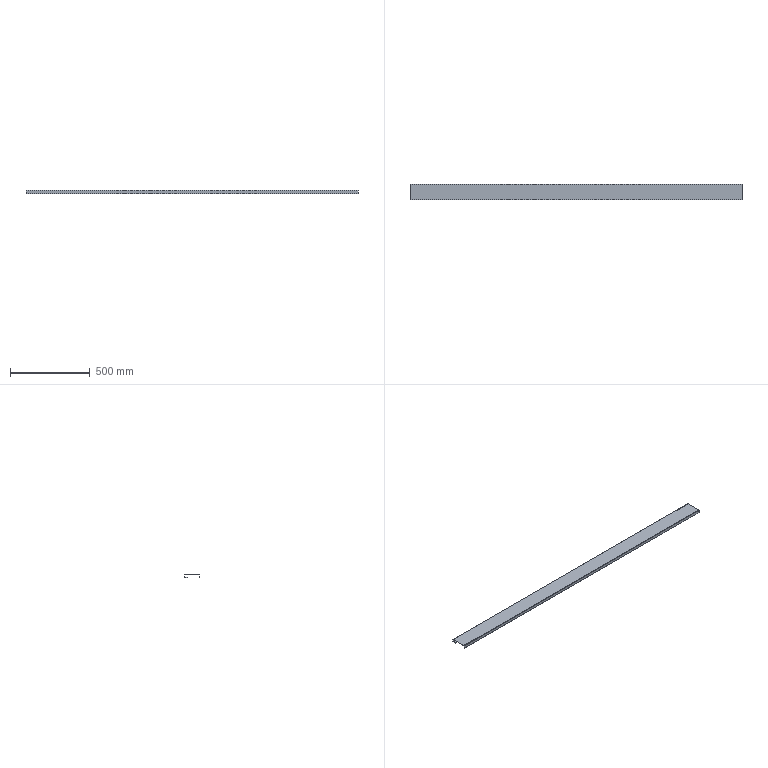Part | STEP file | E3-中转釜护栏3踢脚Plate | 1 solid | 18 faces | box 2088 x 100 x 20 mm | volume 479969 mm3 | plane 12 | cylinder 6 | commonest cylinder face diameters 2 x3 5 x3
STEP:
#1=CARTESIAN_POINT('',(0.,0.,0.));
#2=DIRECTION('',(0.,0.,1.));
#3=DIRECTION('',(1.,0.,0.));
#4=AXIS2_PLACEMENT_3D('',#1,#2,#3);
#5=CARTESIAN_POINT('',(-1044.,1.5,-2.5));
#6=VERTEX_POINT('',#5);
#7=CARTESIAN_POINT('',(-1044.,1.5,-20.));
#8=VERTEX_POINT('',#7);
#9=CARTESIAN_POINT('',(-1044.,1.5,-2.5));
#10=DIRECTION('',(0.,0.,-1.));
#11=VECTOR('',#10,1.);
#12=LINE('',#9,#11);
#13=CARTESIAN_POINT('',(1044.,1.5,-2.5));
#14=DIRECTION('',(0.,-1.,0.));
#15=DIRECTION('',(0.,0.,1.));
#16=AXIS2_PLACEMENT_3D('',#13,#14,#15);
#17=PLANE('',#16);
#18=CARTESIAN_POINT('',(0.,2088.));
#19=DIRECTION('',(-1.,0.));
#20=VECTOR('',#19,1.);
#21=LINE('',#18,#20);
#22=(GEOMETRIC_REPRESENTATION_CONTEXT(2)PARAMETRIC_REPRESENTATION_CONTEXT()REPRESENTATION_CONTEXT('',''));
#23=DEFINITIONAL_REPRESENTATION('',(#21),#22);
#24=PCURVE('',#17,#23);
#25=CARTESIAN_POINT('',(-1044.,2.5,-2.5));
#26=DIRECTION('',(-1.,0.,0.));
#27=DIRECTION('',(0.,0.,-1.));
#28=AXIS2_PLACEMENT_3D('',#25,#26,#27);
#29=PLANE('',#28);
#30=CARTESIAN_POINT('',(0.,1.));
#31=DIRECTION('',(1.,0.));
#32=VECTOR('',#31,1.);
#33=LINE('',#30,#32);
#34=(GEOMETRIC_REPRESENTATION_CONTEXT(2)PARAMETRIC_REPRESENTATION_CONTEXT()REPRESENTATION_CONTEXT('',''));
#35=DEFINITIONAL_REPRESENTATION('',(#33),#34);
#36=PCURVE('',#29,#35);
#37=SURFACE_CURVE('',#12,(#24,#36),.PCURVE_S1.);
#38=EDGE_CURVE('',#6,#8,#37,.T.);
#39=ORIENTED_EDGE('',*,*,#38,.F.);
#40=CARTESIAN_POINT('',(1044.,1.5,-2.5));
#41=VERTEX_POINT('',#40);
#42=CARTESIAN_POINT('',(1044.,1.5,-2.5));
#43=DIRECTION('',(-1.,0.,0.));
#44=VECTOR('',#43,1.);
#45=LINE('',#42,#44);
#46=CARTESIAN_POINT('',(0.,0.));
#47=DIRECTION('',(0.,1.));
#48=VECTOR('',#47,1.);
#49=LINE('',#46,#48);
#50=(GEOMETRIC_REPRESENTATION_CONTEXT(2)PARAMETRIC_REPRESENTATION_CONTEXT()REPRESENTATION_CONTEXT('',''));
#51=DEFINITIONAL_REPRESENTATION('',(#49),#50);
#52=PCURVE('',#17,#51);
#53=CARTESIAN_POINT('',(1044.,2.5,-2.5));
#54=DIRECTION('',(-1.,0.,0.));
#55=DIRECTION('',(0.,0.,-1.));
#56=AXIS2_PLACEMENT_3D('',#53,#54,#55);
#57=CYLINDRICAL_SURFACE('',#56,1.);
#58=CARTESIAN_POINT('',(1.571,0.));
#59=DIRECTION('',(0.,1.));
#60=VECTOR('',#59,1.);
#61=LINE('',#58,#60);
#62=(GEOMETRIC_REPRESENTATION_CONTEXT(2)PARAMETRIC_REPRESENTATION_CONTEXT()REPRESENTATION_CONTEXT('',''));
#63=DEFINITIONAL_REPRESENTATION('',(#61),#62);
#64=PCURVE('',#57,#63);
#65=SURFACE_CURVE('',#45,(#52,#64),.PCURVE_S1.);
#66=EDGE_CURVE('',#41,#6,#65,.T.);
#67=ORIENTED_EDGE('',*,*,#66,.F.);
#68=CARTESIAN_POINT('',(1044.,1.5,-20.));
#69=VERTEX_POINT('',#68);
#70=CARTESIAN_POINT('',(1044.,1.5,-2.5));
#71=DIRECTION('',(0.,0.,-1.));
#72=VECTOR('',#71,1.);
#73=LINE('',#70,#72);
#74=CARTESIAN_POINT('',(0.,0.));
#75=DIRECTION('',(-1.,0.));
#76=VECTOR('',#75,1.);
#77=LINE('',#74,#76);
#78=(GEOMETRIC_REPRESENTATION_CONTEXT(2)PARAMETRIC_REPRESENTATION_CONTEXT()REPRESENTATION_CONTEXT('',''));
#79=DEFINITIONAL_REPRESENTATION('',(#77),#78);
#80=PCURVE('',#17,#79);
#81=CARTESIAN_POINT('',(1044.,2.5,-2.5));
#82=DIRECTION('',(-1.,0.,0.));
#83=DIRECTION('',(0.,0.,-1.));
#84=AXIS2_PLACEMENT_3D('',#81,#82,#83);
#85=PLANE('',#84);
#86=CARTESIAN_POINT('',(0.,1.));
#87=DIRECTION('',(1.,0.));
#88=VECTOR('',#87,1.);
#89=LINE('',#86,#88);
#90=(GEOMETRIC_REPRESENTATION_CONTEXT(2)PARAMETRIC_REPRESENTATION_CONTEXT()REPRESENTATION_CONTEXT('',''));
#91=DEFINITIONAL_REPRESENTATION('',(#89),#90);
#92=PCURVE('',#85,#91);
#93=SURFACE_CURVE('',#73,(#80,#92),.PCURVE_S1.);
#94=EDGE_CURVE('',#41,#69,#93,.T.);
#95=ORIENTED_EDGE('',*,*,#94,.T.);
#96=CARTESIAN_POINT('',(1044.,1.5,-20.));
#97=DIRECTION('',(-1.,0.,0.));
#98=VECTOR('',#97,1.);
#99=LINE('',#96,#98);
#100=CARTESIAN_POINT('',(-17.5,0.));
#101=DIRECTION('',(0.,1.));
#102=VECTOR('',#101,1.);
#103=LINE('',#100,#102);
#104=(GEOMETRIC_REPRESENTATION_CONTEXT(2)PARAMETRIC_REPRESENTATION_CONTEXT()REPRESENTATION_CONTEXT('',''));
#105=DEFINITIONAL_REPRESENTATION('',(#103),#104);
#106=PCURVE('',#17,#105);
#107=CARTESIAN_POINT('',(1044.,0.,-20.));
#108=DIRECTION('',(0.,0.,-1.));
#109=DIRECTION('',(1.,0.,0.));
#110=AXIS2_PLACEMENT_3D('',#107,#108,#109);
#111=PLANE('',#110);
#112=CARTESIAN_POINT('',(0.,-1.5));
#113=DIRECTION('',(-1.,0.));
#114=VECTOR('',#113,1.);
#115=LINE('',#112,#114);
#116=(GEOMETRIC_REPRESENTATION_CONTEXT(2)PARAMETRIC_REPRESENTATION_CONTEXT()REPRESENTATION_CONTEXT('',''));
#117=DEFINITIONAL_REPRESENTATION('',(#115),#116);
#118=PCURVE('',#111,#117);
#119=SURFACE_CURVE('',#99,(#106,#118),.PCURVE_S1.);
#120=EDGE_CURVE('',#69,#8,#119,.T.);
#121=ORIENTED_EDGE('',*,*,#120,.T.);
#122=EDGE_LOOP('',(#39,#67,#95,#121));
#123=FACE_BOUND('',#122,.T.);
#124=ADVANCED_FACE('',(#123),#17,.F.);
#125=CARTESIAN_POINT('',(-1044.,0.,-20.));
#126=VERTEX_POINT('',#125);
#127=CARTESIAN_POINT('',(-1044.,0.,-20.));
#128=DIRECTION('',(0.,1.,0.));
#129=VECTOR('',#128,1.);
#130=LINE('',#127,#129);
#131=CARTESIAN_POINT('',(-2088.,0.));
#132=DIRECTION('',(0.,-1.));
#133=VECTOR('',#132,1.);
#134=LINE('',#131,#133);
#135=(GEOMETRIC_REPRESENTATION_CONTEXT(2)PARAMETRIC_REPRESENTATION_CONTEXT()REPRESENTATION_CONTEXT('',''));
#136=DEFINITIONAL_REPRESENTATION('',(#134),#135);
#137=PCURVE('',#111,#136);
#138=CARTESIAN_POINT('',(17.5,2.5));
#139=DIRECTION('',(0.,-1.));
#140=VECTOR('',#139,1.);
#141=LINE('',#138,#140);
#142=(GEOMETRIC_REPRESENTATION_CONTEXT(2)PARAMETRIC_REPRESENTATION_CONTEXT()REPRESENTATION_CONTEXT('',''));
#143=DEFINITIONAL_REPRESENTATION('',(#141),#142);
#144=PCURVE('',#29,#143);
#145=SURFACE_CURVE('',#130,(#137,#144),.PCURVE_S1.);
#146=EDGE_CURVE('',#126,#8,#145,.T.);
#147=ORIENTED_EDGE('',*,*,#146,.T.);
#148=ORIENTED_EDGE('',*,*,#120,.F.);
#149=CARTESIAN_POINT('',(1044.,0.,-20.));
#150=VERTEX_POINT('',#149);
#151=CARTESIAN_POINT('',(1044.,0.,-20.));
#152=DIRECTION('',(0.,1.,0.));
#153=VECTOR('',#152,1.);
#154=LINE('',#151,#153);
#155=CARTESIAN_POINT('',(0.,0.));
#156=DIRECTION('',(0.,-1.));
#157=VECTOR('',#156,1.);
#158=LINE('',#155,#157);
#159=(GEOMETRIC_REPRESENTATION_CONTEXT(2)PARAMETRIC_REPRESENTATION_CONTEXT()REPRESENTATION_CONTEXT('',''));
#160=DEFINITIONAL_REPRESENTATION('',(#158),#159);
#161=PCURVE('',#111,#160);
#162=CARTESIAN_POINT('',(17.5,2.5));
#163=DIRECTION('',(0.,-1.));
#164=VECTOR('',#163,1.);
#165=LINE('',#162,#164);
#166=(GEOMETRIC_REPRESENTATION_CONTEXT(2)PARAMETRIC_REPRESENTATION_CONTEXT()REPRESENTATION_CONTEXT('',''));
#167=DEFINITIONAL_REPRESENTATION('',(#165),#166);
#168=PCURVE('',#85,#167);
#169=SURFACE_CURVE('',#154,(#161,#168),.PCURVE_S1.);
#170=EDGE_CURVE('',#150,#69,#169,.T.);
#171=ORIENTED_EDGE('',*,*,#170,.F.);
#172=CARTESIAN_POINT('',(1044.,0.,-20.));
#173=DIRECTION('',(-1.,0.,0.));
#174=VECTOR('',#173,1.);
#175=LINE('',#172,#174);
#176=CARTESIAN_POINT('',(0.,0.));
#177=DIRECTION('',(-1.,0.));
#178=VECTOR('',#177,1.);
#179=LINE('',#176,#178);
#180=(GEOMETRIC_REPRESENTATION_CONTEXT(2)PARAMETRIC_REPRESENTATION_CONTEXT()REPRESENTATION_CONTEXT('',''));
#181=DEFINITIONAL_REPRESENTATION('',(#179),#180);
#182=PCURVE('',#111,#181);
#183=CARTESIAN_POINT('',(1044.,0.,-2.5));
#184=DIRECTION('',(0.,-1.,0.));
#185=DIRECTION('',(0.,0.,1.));
#186=AXIS2_PLACEMENT_3D('',#183,#184,#185);
#187=PLANE('',#186);
#188=CARTESIAN_POINT('',(-17.5,0.));
#189=DIRECTION('',(0.,1.));
#190=VECTOR('',#189,1.);
#191=LINE('',#188,#190);
#192=(GEOMETRIC_REPRESENTATION_CONTEXT(2)PARAMETRIC_REPRESENTATION_CONTEXT()REPRESENTATION_CONTEXT('',''));
#193=DEFINITIONAL_REPRESENTATION('',(#191),#192);
#194=PCURVE('',#187,#193);
#195=SURFACE_CURVE('',#175,(#182,#194),.PCURVE_S1.);
#196=EDGE_CURVE('',#150,#126,#195,.T.);
#197=ORIENTED_EDGE('',*,*,#196,.T.);
#198=EDGE_LOOP('',(#147,#148,#171,#197));
#199=FACE_BOUND('',#198,.T.);
#200=ADVANCED_FACE('',(#199),#111,.T.);
#201=CARTESIAN_POINT('',(-1044.,0.,-2.5));
#202=VERTEX_POINT('',#201);
#203=CARTESIAN_POINT('',(-1044.,0.,-2.5));
#204=DIRECTION('',(0.,0.,-1.));
#205=VECTOR('',#204,1.);
#206=LINE('',#203,#205);
#207=CARTESIAN_POINT('',(0.,2088.));
#208=DIRECTION('',(-1.,0.));
#209=VECTOR('',#208,1.);
#210=LINE('',#207,#209);
#211=(GEOMETRIC_REPRESENTATION_CONTEXT(2)PARAMETRIC_REPRESENTATION_CONTEXT()REPRESENTATION_CONTEXT('',''));
#212=DEFINITIONAL_REPRESENTATION('',(#210),#211);
#213=PCURVE('',#187,#212);
#214=CARTESIAN_POINT('',(0.,2.5));
#215=DIRECTION('',(1.,0.));
#216=VECTOR('',#215,1.);
#217=LINE('',#214,#216);
#218=(GEOMETRIC_REPRESENTATION_CONTEXT(2)PARAMETRIC_REPRESENTATION_CONTEXT()REPRESENTATION_CONTEXT('',''));
#219=DEFINITIONAL_REPRESENTATION('',(#217),#218);
#220=PCURVE('',#29,#219);
#221=SURFACE_CURVE('',#206,(#213,#220),.PCURVE_S1.);
#222=EDGE_CURVE('',#202,#126,#221,.T.);
#223=ORIENTED_EDGE('',*,*,#222,.T.);
#224=ORIENTED_EDGE('',*,*,#196,.F.);
#225=CARTESIAN_POINT('',(1044.,0.,-2.5));
#226=VERTEX_POINT('',#225);
#227=CARTESIAN_POINT('',(1044.,0.,-2.5));
#228=DIRECTION('',(0.,0.,-1.));
#229=VECTOR('',#228,1.);
#230=LINE('',#227,#229);
#231=CARTESIAN_POINT('',(0.,0.));
#232=DIRECTION('',(-1.,0.));
#233=VECTOR('',#232,1.);
#234=LINE('',#231,#233);
#235=(GEOMETRIC_REPRESENTATION_CONTEXT(2)PARAMETRIC_REPRESENTATION_CONTEXT()REPRESENTATION_CONTEXT('',''));
#236=DEFINITIONAL_REPRESENTATION('',(#234),#235);
#237=PCURVE('',#187,#236);
#238=CARTESIAN_POINT('',(0.,2.5));
#239=DIRECTION('',(1.,0.));
#240=VECTOR('',#239,1.);
#241=LINE('',#238,#240);
#242=(GEOMETRIC_REPRESENTATION_CONTEXT(2)PARAMETRIC_REPRESENTATION_CONTEXT()REPRESENTATION_CONTEXT('',''));
#243=DEFINITIONAL_REPRESENTATION('',(#241),#242);
#244=PCURVE('',#85,#243);
#245=SURFACE_CURVE('',#230,(#237,#244),.PCURVE_S1.);
#246=EDGE_CURVE('',#226,#150,#245,.T.);
#247=ORIENTED_EDGE('',*,*,#246,.F.);
#248=CARTESIAN_POINT('',(1044.,0.,-2.5));
#249=DIRECTION('',(-1.,0.,0.));
#250=VECTOR('',#249,1.);
#251=LINE('',#248,#250);
#252=CARTESIAN_POINT('',(0.,0.));
#253=DIRECTION('',(0.,1.));
#254=VECTOR('',#253,1.);
#255=LINE('',#252,#254);
#256=(GEOMETRIC_REPRESENTATION_CONTEXT(2)PARAMETRIC_REPRESENTATION_CONTEXT()REPRESENTATION_CONTEXT('',''));
#257=DEFINITIONAL_REPRESENTATION('',(#255),#256);
#258=PCURVE('',#187,#257);
#259=CARTESIAN_POINT('',(1044.,2.5,-2.5));
#260=DIRECTION('',(-1.,0.,0.));
#261=DIRECTION('',(0.,0.,-1.));
#262=AXIS2_PLACEMENT_3D('',#259,#260,#261);
#263=CYLINDRICAL_SURFACE('',#262,2.5);
#264=CARTESIAN_POINT('',(1.571,0.));
#265=DIRECTION('',(0.,1.));
#266=VECTOR('',#265,1.);
#267=LINE('',#264,#266);
#268=(GEOMETRIC_REPRESENTATION_CONTEXT(2)PARAMETRIC_REPRESENTATION_CONTEXT()REPRESENTATION_CONTEXT('',''));
#269=DEFINITIONAL_REPRESENTATION('',(#267),#268);
#270=PCURVE('',#263,#269);
#271=SURFACE_CURVE('',#251,(#258,#270),.PCURVE_S1.);
#272=EDGE_CURVE('',#226,#202,#271,.T.);
#273=ORIENTED_EDGE('',*,*,#272,.T.);
#274=EDGE_LOOP('',(#223,#224,#247,#273));
#275=FACE_BOUND('',#274,.T.);
#276=ADVANCED_FACE('',(#275),#187,.T.);
#277=CARTESIAN_POINT('',(-1044.,2.5,0.));
#278=VERTEX_POINT('',#277);
#279=CARTESIAN_POINT('',(-1044.,2.5,-2.5));
#280=DIRECTION('',(1.,0.,0.));
#281=DIRECTION('',(0.,0.,-1.));
#282=AXIS2_PLACEMENT_3D('',#279,#280,#281);
#283=CIRCLE('',#282,2.5);
#284=CARTESIAN_POINT('',(6.283,2088.));
#285=DIRECTION('',(-1.,0.));
#286=VECTOR('',#285,1.);
#287=LINE('',#284,#286);
#288=(GEOMETRIC_REPRESENTATION_CONTEXT(2)PARAMETRIC_REPRESENTATION_CONTEXT()REPRESENTATION_CONTEXT('',''));
#289=DEFINITIONAL_REPRESENTATION('',(#287),#288);
#290=PCURVE('',#263,#289);
#291=CARTESIAN_POINT('',(2.5,0.));
#292=CARTESIAN_POINT('',(2.5,-4.33));
#293=CARTESIAN_POINT('',(-1.25,-2.165));
#294=CARTESIAN_POINT('',(-5.,0.));
#295=CARTESIAN_POINT('',(-1.25,2.165));
#296=CARTESIAN_POINT('',(2.5,4.33));
#297=CARTESIAN_POINT('',(2.5,0.));
#298=(BOUNDED_CURVE()B_SPLINE_CURVE(2,(#291,#292,#293,#294,#295,#296,#297),.UNSPECIFIED.,.T.,.F.)B_SPLINE_CURVE_WITH_KNOTS((1,2,2,2,2,1),(-2.094,0.,2.094,4.189,6.283,8.378),.UNSPECIFIED.)CURVE()GEOMETRIC_REPRESENTATION_ITEM()RATIONAL_B_SPLINE_CURVE((1.,0.5,1.,0.5,1.,0.5,1.))REPRESENTATION_ITEM(''));
#299=(GEOMETRIC_REPRESENTATION_CONTEXT(2)PARAMETRIC_REPRESENTATION_CONTEXT()REPRESENTATION_CONTEXT('',''));
#300=DEFINITIONAL_REPRESENTATION('',(#298),#299);
#301=PCURVE('',#29,#300);
#302=SURFACE_CURVE('',#283,(#290,#301),.PCURVE_S1.);
#303=EDGE_CURVE('',#278,#202,#302,.T.);
#304=ORIENTED_EDGE('',*,*,#303,.T.);
#305=ORIENTED_EDGE('',*,*,#272,.F.);
#306=CARTESIAN_POINT('',(1044.,2.5,0.));
#307=VERTEX_POINT('',#306);
#308=CARTESIAN_POINT('',(1044.,2.5,-2.5));
#309=DIRECTION('',(1.,0.,0.));
#310=DIRECTION('',(0.,0.,-1.));
#311=AXIS2_PLACEMENT_3D('',#308,#309,#310);
#312=CIRCLE('',#311,2.5);
#313=CARTESIAN_POINT('',(6.283,0.));
#314=DIRECTION('',(-1.,0.));
#315=VECTOR('',#314,1.);
#316=LINE('',#313,#315);
#317=(GEOMETRIC_REPRESENTATION_CONTEXT(2)PARAMETRIC_REPRESENTATION_CONTEXT()REPRESENTATION_CONTEXT('',''));
#318=DEFINITIONAL_REPRESENTATION('',(#316),#317);
#319=PCURVE('',#263,#318);
#320=CARTESIAN_POINT('',(2.5,0.));
#321=CARTESIAN_POINT('',(2.5,-4.33));
#322=CARTESIAN_POINT('',(-1.25,-2.165));
#323=CARTESIAN_POINT('',(-5.,0.));
#324=CARTESIAN_POINT('',(-1.25,2.165));
#325=CARTESIAN_POINT('',(2.5,4.33));
#326=CARTESIAN_POINT('',(2.5,0.));
#327=(BOUNDED_CURVE()B_SPLINE_CURVE(2,(#320,#321,#322,#323,#324,#325,#326),.UNSPECIFIED.,.T.,.F.)B_SPLINE_CURVE_WITH_KNOTS((1,2,2,2,2,1),(-2.094,0.,2.094,4.189,6.283,8.378),.UNSPECIFIED.)CURVE()GEOMETRIC_REPRESENTATION_ITEM()RATIONAL_B_SPLINE_CURVE((1.,0.5,1.,0.5,1.,0.5,1.))REPRESENTATION_ITEM(''));
#328=(GEOMETRIC_REPRESENTATION_CONTEXT(2)PARAMETRIC_REPRESENTATION_CONTEXT()REPRESENTATION_CONTEXT('',''));
#329=DEFINITIONAL_REPRESENTATION('',(#327),#328);
#330=PCURVE('',#85,#329);
#331=SURFACE_CURVE('',#312,(#319,#330),.PCURVE_S1.);
#332=EDGE_CURVE('',#307,#226,#331,.T.);
#333=ORIENTED_EDGE('',*,*,#332,.F.);
#334=CARTESIAN_POINT('',(1044.,2.5,0.));
#335=DIRECTION('',(-1.,0.,0.));
#336=VECTOR('',#335,1.);
#337=LINE('',#334,#336);
#338=CARTESIAN_POINT('',(3.142,0.));
#339=DIRECTION('',(0.,1.));
#340=VECTOR('',#339,1.);
#341=LINE('',#338,#340);
#342=(GEOMETRIC_REPRESENTATION_CONTEXT(2)PARAMETRIC_REPRESENTATION_CONTEXT()REPRESENTATION_CONTEXT('',''));
#343=DEFINITIONAL_REPRESENTATION('',(#341),#342);
#344=PCURVE('',#263,#343);
#345=CARTESIAN_POINT('',(1044.,2.5,0.));
#346=DIRECTION('',(0.,0.,1.));
#347=DIRECTION('',(-1.,0.,0.));
#348=AXIS2_PLACEMENT_3D('',#345,#346,#347);
#349=PLANE('',#348);
#350=CARTESIAN_POINT('',(0.,0.));
#351=DIRECTION('',(1.,0.));
#352=VECTOR('',#351,1.);
#353=LINE('',#350,#352);
#354=(GEOMETRIC_REPRESENTATION_CONTEXT(2)PARAMETRIC_REPRESENTATION_CONTEXT()REPRESENTATION_CONTEXT('',''));
#355=DEFINITIONAL_REPRESENTATION('',(#353),#354);
#356=PCURVE('',#349,#355);
#357=SURFACE_CURVE('',#337,(#344,#356),.PCURVE_S1.);
#358=EDGE_CURVE('',#307,#278,#357,.T.);
#359=ORIENTED_EDGE('',*,*,#358,.T.);
#360=EDGE_LOOP('',(#304,#305,#333,#359));
#361=FACE_BOUND('',#360,.T.);
#362=ADVANCED_FACE('',(#361),#263,.T.);
#363=CARTESIAN_POINT('',(-1044.,97.5,0.));
#364=VERTEX_POINT('',#363);
#365=CARTESIAN_POINT('',(-1044.,2.5,0.));
#366=DIRECTION('',(0.,-1.,0.));
#367=VECTOR('',#366,1.);
#368=LINE('',#365,#367);
#369=CARTESIAN_POINT('',(2088.,0.));
#370=DIRECTION('',(0.,1.));
#371=VECTOR('',#370,1.);
#372=LINE('',#369,#371);
#373=(GEOMETRIC_REPRESENTATION_CONTEXT(2)PARAMETRIC_REPRESENTATION_CONTEXT()REPRESENTATION_CONTEXT('',''));
#374=DEFINITIONAL_REPRESENTATION('',(#372),#373);
#375=PCURVE('',#349,#374);
#376=CARTESIAN_POINT('',(-2.5,0.));
#377=DIRECTION('',(0.,1.));
#378=VECTOR('',#377,1.);
#379=LINE('',#376,#378);
#380=(GEOMETRIC_REPRESENTATION_CONTEXT(2)PARAMETRIC_REPRESENTATION_CONTEXT()REPRESENTATION_CONTEXT('',''));
#381=DEFINITIONAL_REPRESENTATION('',(#379),#380);
#382=PCURVE('',#29,#381);
#383=SURFACE_CURVE('',#368,(#375,#382),.PCURVE_S1.);
#384=EDGE_CURVE('',#364,#278,#383,.T.);
#385=ORIENTED_EDGE('',*,*,#384,.T.);
#386=ORIENTED_EDGE('',*,*,#358,.F.);
#387=CARTESIAN_POINT('',(1044.,97.5,0.));
#388=VERTEX_POINT('',#387);
#389=CARTESIAN_POINT('',(1044.,2.5,0.));
#390=DIRECTION('',(0.,-1.,0.));
#391=VECTOR('',#390,1.);
#392=LINE('',#389,#391);
#393=CARTESIAN_POINT('',(0.,0.));
#394=DIRECTION('',(0.,1.));
#395=VECTOR('',#394,1.);
#396=LINE('',#393,#395);
#397=(GEOMETRIC_REPRESENTATION_CONTEXT(2)PARAMETRIC_REPRESENTATION_CONTEXT()REPRESENTATION_CONTEXT('',''));
#398=DEFINITIONAL_REPRESENTATION('',(#396),#397);
#399=PCURVE('',#349,#398);
#400=CARTESIAN_POINT('',(-2.5,0.));
#401=DIRECTION('',(0.,1.));
#402=VECTOR('',#401,1.);
#403=LINE('',#400,#402);
#404=(GEOMETRIC_REPRESENTATION_CONTEXT(2)PARAMETRIC_REPRESENTATION_CONTEXT()REPRESENTATION_CONTEXT('',''));
#405=DEFINITIONAL_REPRESENTATION('',(#403),#404);
#406=PCURVE('',#85,#405);
#407=SURFACE_CURVE('',#392,(#399,#406),.PCURVE_S1.);
#408=EDGE_CURVE('',#388,#307,#407,.T.);
#409=ORIENTED_EDGE('',*,*,#408,.F.);
#410=CARTESIAN_POINT('',(1044.,97.5,0.));
#411=DIRECTION('',(-1.,0.,0.));
#412=VECTOR('',#411,1.);
#413=LINE('',#410,#412);
#414=CARTESIAN_POINT('',(0.,-95.));
#415=DIRECTION('',(1.,0.));
#416=VECTOR('',#415,1.);
#417=LINE('',#414,#416);
#418=(GEOMETRIC_REPRESENTATION_CONTEXT(2)PARAMETRIC_REPRESENTATION_CONTEXT()REPRESENTATION_CONTEXT('',''));
#419=DEFINITIONAL_REPRESENTATION('',(#417),#418);
#420=PCURVE('',#349,#419);
#421=CARTESIAN_POINT('',(1044.,97.5,-2.5));
#422=DIRECTION('',(-1.,0.,0.));
#423=DIRECTION('',(0.,0.,-1.));
#424=AXIS2_PLACEMENT_3D('',#421,#422,#423);
#425=CYLINDRICAL_SURFACE('',#424,2.5);
#426=CARTESIAN_POINT('',(3.142,0.));
#427=DIRECTION('',(0.,1.));
#428=VECTOR('',#427,1.);
#429=LINE('',#426,#428);
#430=(GEOMETRIC_REPRESENTATION_CONTEXT(2)PARAMETRIC_REPRESENTATION_CONTEXT()REPRESENTATION_CONTEXT('',''));
#431=DEFINITIONAL_REPRESENTATION('',(#429),#430);
#432=PCURVE('',#425,#431);
#433=SURFACE_CURVE('',#413,(#420,#432),.PCURVE_S1.);
#434=EDGE_CURVE('',#388,#364,#433,.T.);
#435=ORIENTED_EDGE('',*,*,#434,.T.);
#436=EDGE_LOOP('',(#385,#386,#409,#435));
#437=FACE_BOUND('',#436,.T.);
#438=ADVANCED_FACE('',(#437),#349,.T.);
#439=CARTESIAN_POINT('',(-1044.,100.,-2.5));
#440=VERTEX_POINT('',#439);
#441=CARTESIAN_POINT('',(-1044.,97.5,-2.5));
#442=DIRECTION('',(1.,0.,0.));
#443=DIRECTION('',(0.,0.,1.));
#444=AXIS2_PLACEMENT_3D('',#441,#442,#443);
#445=CIRCLE('',#444,2.5);
#446=CARTESIAN_POINT('',(9.425,2088.));
#447=DIRECTION('',(-1.,0.));
#448=VECTOR('',#447,1.);
#449=LINE('',#446,#448);
#450=(GEOMETRIC_REPRESENTATION_CONTEXT(2)PARAMETRIC_REPRESENTATION_CONTEXT()REPRESENTATION_CONTEXT('',''));
#451=DEFINITIONAL_REPRESENTATION('',(#449),#450);
#452=PCURVE('',#425,#451);
#453=CARTESIAN_POINT('',(-2.5,-95.));
#454=CARTESIAN_POINT('',(-2.5,-90.67));
#455=CARTESIAN_POINT('',(1.25,-92.835));
#456=CARTESIAN_POINT('',(5.,-95.));
#457=CARTESIAN_POINT('',(1.25,-97.165));
#458=CARTESIAN_POINT('',(-2.5,-99.33));
#459=CARTESIAN_POINT('',(-2.5,-95.));
#460=(BOUNDED_CURVE()B_SPLINE_CURVE(2,(#453,#454,#455,#456,#457,#458,#459),.UNSPECIFIED.,.T.,.F.)B_SPLINE_CURVE_WITH_KNOTS((1,2,2,2,2,1),(-2.094,0.,2.094,4.189,6.283,8.378),.UNSPECIFIED.)CURVE()GEOMETRIC_REPRESENTATION_ITEM()RATIONAL_B_SPLINE_CURVE((1.,0.5,1.,0.5,1.,0.5,1.))REPRESENTATION_ITEM(''));
#461=(GEOMETRIC_REPRESENTATION_CONTEXT(2)PARAMETRIC_REPRESENTATION_CONTEXT()REPRESENTATION_CONTEXT('',''));
#462=DEFINITIONAL_REPRESENTATION('',(#460),#461);
#463=PCURVE('',#29,#462);
#464=SURFACE_CURVE('',#445,(#452,#463),.PCURVE_S1.);
#465=EDGE_CURVE('',#440,#364,#464,.T.);
#466=ORIENTED_EDGE('',*,*,#465,.T.);
#467=ORIENTED_EDGE('',*,*,#434,.F.);
#468=CARTESIAN_POINT('',(1044.,100.,-2.5));
#469=VERTEX_POINT('',#468);
#470=CARTESIAN_POINT('',(1044.,97.5,-2.5));
#471=DIRECTION('',(1.,0.,0.));
#472=DIRECTION('',(0.,0.,1.));
#473=AXIS2_PLACEMENT_3D('',#470,#471,#472);
#474=CIRCLE('',#473,2.5);
#475=CARTESIAN_POINT('',(9.425,0.));
#476=DIRECTION('',(-1.,0.));
#477=VECTOR('',#476,1.);
#478=LINE('',#475,#477);
#479=(GEOMETRIC_REPRESENTATION_CONTEXT(2)PARAMETRIC_REPRESENTATION_CONTEXT()REPRESENTATION_CONTEXT('',''));
#480=DEFINITIONAL_REPRESENTATION('',(#478),#479);
#481=PCURVE('',#425,#480);
#482=CARTESIAN_POINT('',(-2.5,-95.));
#483=CARTESIAN_POINT('',(-2.5,-90.67));
#484=CARTESIAN_POINT('',(1.25,-92.835));
#485=CARTESIAN_POINT('',(5.,-95.));
#486=CARTESIAN_POINT('',(1.25,-97.165));
#487=CARTESIAN_POINT('',(-2.5,-99.33));
#488=CARTESIAN_POINT('',(-2.5,-95.));
#489=(BOUNDED_CURVE()B_SPLINE_CURVE(2,(#482,#483,#484,#485,#486,#487,#488),.UNSPECIFIED.,.T.,.F.)B_SPLINE_CURVE_WITH_KNOTS((1,2,2,2,2,1),(-2.094,0.,2.094,4.189,6.283,8.378),.UNSPECIFIED.)CURVE()GEOMETRIC_REPRESENTATION_ITEM()RATIONAL_B_SPLINE_CURVE((1.,0.5,1.,0.5,1.,0.5,1.))REPRESENTATION_ITEM(''));
#490=(GEOMETRIC_REPRESENTATION_CONTEXT(2)PARAMETRIC_REPRESENTATION_CONTEXT()REPRESENTATION_CONTEXT('',''));
#491=DEFINITIONAL_REPRESENTATION('',(#489),#490);
#492=PCURVE('',#85,#491);
#493=SURFACE_CURVE('',#474,(#481,#492),.PCURVE_S1.);
#494=EDGE_CURVE('',#469,#388,#493,.T.);
#495=ORIENTED_EDGE('',*,*,#494,.F.);
#496=CARTESIAN_POINT('',(1044.,100.,-2.5));
#497=DIRECTION('',(-1.,0.,0.));
#498=VECTOR('',#497,1.);
#499=LINE('',#496,#498);
#500=CARTESIAN_POINT('',(4.712,0.));
#501=DIRECTION('',(0.,1.));
#502=VECTOR('',#501,1.);
#503=LINE('',#500,#502);
#504=(GEOMETRIC_REPRESENTATION_CONTEXT(2)PARAMETRIC_REPRESENTATION_CONTEXT()REPRESENTATION_CONTEXT('',''));
#505=DEFINITIONAL_REPRESENTATION('',(#503),#504);
#506=PCURVE('',#425,#505);
#507=CARTESIAN_POINT('',(1044.,100.,-2.5));
#508=DIRECTION('',(0.,1.,0.));
#509=DIRECTION('',(0.,0.,-1.));
#510=AXIS2_PLACEMENT_3D('',#507,#508,#509);
#511=PLANE('',#510);
#512=CARTESIAN_POINT('',(0.,0.));
#513=DIRECTION('',(0.,1.));
#514=VECTOR('',#513,1.);
#515=LINE('',#512,#514);
#516=(GEOMETRIC_REPRESENTATION_CONTEXT(2)PARAMETRIC_REPRESENTATION_CONTEXT()REPRESENTATION_CONTEXT('',''));
#517=DEFINITIONAL_REPRESENTATION('',(#515),#516);
#518=PCURVE('',#511,#517);
#519=SURFACE_CURVE('',#499,(#506,#518),.PCURVE_S1.);
#520=EDGE_CURVE('',#469,#440,#519,.T.);
#521=ORIENTED_EDGE('',*,*,#520,.T.);
#522=EDGE_LOOP('',(#466,#467,#495,#521));
#523=FACE_BOUND('',#522,.T.);
#524=ADVANCED_FACE('',(#523),#425,.T.);
#525=CARTESIAN_POINT('',(-1044.,100.,-17.5));
#526=VERTEX_POINT('',#525);
#527=CARTESIAN_POINT('',(-1044.,100.,-2.5));
#528=DIRECTION('',(0.,0.,1.));
#529=VECTOR('',#528,1.);
#530=LINE('',#527,#529);
#531=CARTESIAN_POINT('',(0.,2088.));
#532=DIRECTION('',(-1.,0.));
#533=VECTOR('',#532,1.);
#534=LINE('',#531,#533);
#535=(GEOMETRIC_REPRESENTATION_CONTEXT(2)PARAMETRIC_REPRESENTATION_CONTEXT()REPRESENTATION_CONTEXT('',''));
#536=DEFINITIONAL_REPRESENTATION('',(#534),#535);
#537=PCURVE('',#511,#536);
#538=CARTESIAN_POINT('',(0.,-97.5));
#539=DIRECTION('',(-1.,0.));
#540=VECTOR('',#539,1.);
#541=LINE('',#538,#540);
#542=(GEOMETRIC_REPRESENTATION_CONTEXT(2)PARAMETRIC_REPRESENTATION_CONTEXT()REPRESENTATION_CONTEXT('',''));
#543=DEFINITIONAL_REPRESENTATION('',(#541),#542);
#544=PCURVE('',#29,#543);
#545=SURFACE_CURVE('',#530,(#537,#544),.PCURVE_S1.);
#546=EDGE_CURVE('',#526,#440,#545,.T.);
#547=ORIENTED_EDGE('',*,*,#546,.T.);
#548=ORIENTED_EDGE('',*,*,#520,.F.);
#549=CARTESIAN_POINT('',(1044.,100.,-17.5));
#550=VERTEX_POINT('',#549);
#551=CARTESIAN_POINT('',(1044.,100.,-2.5));
#552=DIRECTION('',(0.,0.,1.));
#553=VECTOR('',#552,1.);
#554=LINE('',#551,#553);
#555=CARTESIAN_POINT('',(0.,0.));
#556=DIRECTION('',(-1.,0.));
#557=VECTOR('',#556,1.);
#558=LINE('',#555,#557);
#559=(GEOMETRIC_REPRESENTATION_CONTEXT(2)PARAMETRIC_REPRESENTATION_CONTEXT()REPRESENTATION_CONTEXT('',''));
#560=DEFINITIONAL_REPRESENTATION('',(#558),#559);
#561=PCURVE('',#511,#560);
#562=CARTESIAN_POINT('',(0.,-97.5));
#563=DIRECTION('',(-1.,0.));
#564=VECTOR('',#563,1.);
#565=LINE('',#562,#564);
#566=(GEOMETRIC_REPRESENTATION_CONTEXT(2)PARAMETRIC_REPRESENTATION_CONTEXT()REPRESENTATION_CONTEXT('',''));
#567=DEFINITIONAL_REPRESENTATION('',(#565),#566);
#568=PCURVE('',#85,#567);
#569=SURFACE_CURVE('',#554,(#561,#568),.PCURVE_S1.);
#570=EDGE_CURVE('',#550,#469,#569,.T.);
#571=ORIENTED_EDGE('',*,*,#570,.F.);
#572=CARTESIAN_POINT('',(1044.,100.,-17.5));
#573=DIRECTION('',(-1.,0.,0.));
#574=VECTOR('',#573,1.);
#575=LINE('',#572,#574);
#576=CARTESIAN_POINT('',(15.,0.));
#577=DIRECTION('',(0.,1.));
#578=VECTOR('',#577,1.);
#579=LINE('',#576,#578);
#580=(GEOMETRIC_REPRESENTATION_CONTEXT(2)PARAMETRIC_REPRESENTATION_CONTEXT()REPRESENTATION_CONTEXT('',''));
#581=DEFINITIONAL_REPRESENTATION('',(#579),#580);
#582=PCURVE('',#511,#581);
#583=CARTESIAN_POINT('',(1044.,97.5,-17.5));
#584=DIRECTION('',(-1.,0.,0.));
#585=DIRECTION('',(0.,0.,-1.));
#586=AXIS2_PLACEMENT_3D('',#583,#584,#585);
#587=CYLINDRICAL_SURFACE('',#586,2.5);
#588=CARTESIAN_POINT('',(4.712,0.));
#589=DIRECTION('',(0.,1.));
#590=VECTOR('',#589,1.);
#591=LINE('',#588,#590);
#592=(GEOMETRIC_REPRESENTATION_CONTEXT(2)PARAMETRIC_REPRESENTATION_CONTEXT()REPRESENTATION_CONTEXT('',''));
#593=DEFINITIONAL_REPRESENTATION('',(#591),#592);
#594=PCURVE('',#587,#593);
#595=SURFACE_CURVE('',#575,(#582,#594),.PCURVE_S1.);
#596=EDGE_CURVE('',#550,#526,#595,.T.);
#597=ORIENTED_EDGE('',*,*,#596,.T.);
#598=EDGE_LOOP('',(#547,#548,#571,#597));
#599=FACE_BOUND('',#598,.T.);
#600=ADVANCED_FACE('',(#599),#511,.T.);
#601=CARTESIAN_POINT('',(-1044.,97.5,-20.));
#602=VERTEX_POINT('',#601);
#603=CARTESIAN_POINT('',(-1044.,97.5,-17.5));
#604=DIRECTION('',(1.,0.,0.));
#605=DIRECTION('',(0.,0.,1.));
#606=AXIS2_PLACEMENT_3D('',#603,#604,#605);
#607=CIRCLE('',#606,2.5);
#608=CARTESIAN_POINT('',(9.425,2088.));
#609=DIRECTION('',(-1.,0.));
#610=VECTOR('',#609,1.);
#611=LINE('',#608,#610);
#612=(GEOMETRIC_REPRESENTATION_CONTEXT(2)PARAMETRIC_REPRESENTATION_CONTEXT()REPRESENTATION_CONTEXT('',''));
#613=DEFINITIONAL_REPRESENTATION('',(#611),#612);
#614=PCURVE('',#587,#613);
#615=CARTESIAN_POINT('',(12.5,-95.));
#616=CARTESIAN_POINT('',(12.5,-90.67));
#617=CARTESIAN_POINT('',(16.25,-92.835));
#618=CARTESIAN_POINT('',(20.,-95.));
#619=CARTESIAN_POINT('',(16.25,-97.165));
#620=CARTESIAN_POINT('',(12.5,-99.33));
#621=CARTESIAN_POINT('',(12.5,-95.));
#622=(BOUNDED_CURVE()B_SPLINE_CURVE(2,(#615,#616,#617,#618,#619,#620,#621),.UNSPECIFIED.,.T.,.F.)B_SPLINE_CURVE_WITH_KNOTS((1,2,2,2,2,1),(-2.094,0.,2.094,4.189,6.283,8.378),.UNSPECIFIED.)CURVE()GEOMETRIC_REPRESENTATION_ITEM()RATIONAL_B_SPLINE_CURVE((1.,0.5,1.,0.5,1.,0.5,1.))REPRESENTATION_ITEM(''));
#623=(GEOMETRIC_REPRESENTATION_CONTEXT(2)PARAMETRIC_REPRESENTATION_CONTEXT()REPRESENTATION_CONTEXT('',''));
#624=DEFINITIONAL_REPRESENTATION('',(#622),#623);
#625=PCURVE('',#29,#624);
#626=SURFACE_CURVE('',#607,(#614,#625),.PCURVE_S1.);
#627=EDGE_CURVE('',#602,#526,#626,.T.);
#628=ORIENTED_EDGE('',*,*,#627,.T.);
#629=ORIENTED_EDGE('',*,*,#596,.F.);
#630=CARTESIAN_POINT('',(1044.,97.5,-20.));
#631=VERTEX_POINT('',#630);
#632=CARTESIAN_POINT('',(1044.,97.5,-17.5));
#633=DIRECTION('',(1.,0.,0.));
#634=DIRECTION('',(0.,0.,1.));
#635=AXIS2_PLACEMENT_3D('',#632,#633,#634);
#636=CIRCLE('',#635,2.5);
#637=CARTESIAN_POINT('',(9.425,0.));
#638=DIRECTION('',(-1.,0.));
#639=VECTOR('',#638,1.);
#640=LINE('',#637,#639);
#641=(GEOMETRIC_REPRESENTATION_CONTEXT(2)PARAMETRIC_REPRESENTATION_CONTEXT()REPRESENTATION_CONTEXT('',''));
#642=DEFINITIONAL_REPRESENTATION('',(#640),#641);
#643=PCURVE('',#587,#642);
#644=CARTESIAN_POINT('',(12.5,-95.));
#645=CARTESIAN_POINT('',(12.5,-90.67));
#646=CARTESIAN_POINT('',(16.25,-92.835));
#647=CARTESIAN_POINT('',(20.,-95.));
#648=CARTESIAN_POINT('',(16.25,-97.165));
#649=CARTESIAN_POINT('',(12.5,-99.33));
#650=CARTESIAN_POINT('',(12.5,-95.));
#651=(BOUNDED_CURVE()B_SPLINE_CURVE(2,(#644,#645,#646,#647,#648,#649,#650),.UNSPECIFIED.,.T.,.F.)B_SPLINE_CURVE_WITH_KNOTS((1,2,2,2,2,1),(-2.094,0.,2.094,4.189,6.283,8.378),.UNSPECIFIED.)CURVE()GEOMETRIC_REPRESENTATION_ITEM()RATIONAL_B_SPLINE_CURVE((1.,0.5,1.,0.5,1.,0.5,1.))REPRESENTATION_ITEM(''));
#652=(GEOMETRIC_REPRESENTATION_CONTEXT(2)PARAMETRIC_REPRESENTATION_CONTEXT()REPRESENTATION_CONTEXT('',''));
#653=DEFINITIONAL_REPRESENTATION('',(#651),#652);
#654=PCURVE('',#85,#653);
#655=SURFACE_CURVE('',#636,(#643,#654),.PCURVE_S1.);
#656=EDGE_CURVE('',#631,#550,#655,.T.);
#657=ORIENTED_EDGE('',*,*,#656,.F.);
#658=CARTESIAN_POINT('',(1044.,97.5,-20.));
#659=DIRECTION('',(-1.,0.,0.));
#660=VECTOR('',#659,1.);
#661=LINE('',#658,#660);
#662=CARTESIAN_POINT('',(6.283,0.));
#663=DIRECTION('',(0.,1.));
#664=VECTOR('',#663,1.);
#665=LINE('',#662,#664);
#666=(GEOMETRIC_REPRESENTATION_CONTEXT(2)PARAMETRIC_REPRESENTATION_CONTEXT()REPRESENTATION_CONTEXT('',''));
#667=DEFINITIONAL_REPRESENTATION('',(#665),#666);
#668=PCURVE('',#587,#667);
#669=CARTESIAN_POINT('',(1044.,97.5,-20.));
#670=DIRECTION('',(0.,0.,-1.));
#671=DIRECTION('',(1.,0.,0.));
#672=AXIS2_PLACEMENT_3D('',#669,#670,#671);
#673=PLANE('',#672);
#674=CARTESIAN_POINT('',(0.,0.));
#675=DIRECTION('',(-1.,0.));
#676=VECTOR('',#675,1.);
#677=LINE('',#674,#676);
#678=(GEOMETRIC_REPRESENTATION_CONTEXT(2)PARAMETRIC_REPRESENTATION_CONTEXT()REPRESENTATION_CONTEXT('',''));
#679=DEFINITIONAL_REPRESENTATION('',(#677),#678);
#680=PCURVE('',#673,#679);
#681=SURFACE_CURVE('',#661,(#668,#680),.PCURVE_S1.);
#682=EDGE_CURVE('',#631,#602,#681,.T.);
#683=ORIENTED_EDGE('',*,*,#682,.T.);
#684=EDGE_LOOP('',(#628,#629,#657,#683));
#685=FACE_BOUND('',#684,.T.);
#686=ADVANCED_FACE('',(#685),#587,.T.);
#687=CARTESIAN_POINT('',(-1044.,80.,-20.));
#688=VERTEX_POINT('',#687);
#689=CARTESIAN_POINT('',(-1044.,97.5,-20.));
#690=DIRECTION('',(0.,1.,0.));
#691=VECTOR('',#690,1.);
#692=LINE('',#689,#691);
#693=CARTESIAN_POINT('',(-2088.,0.));
#694=DIRECTION('',(0.,-1.));
#695=VECTOR('',#694,1.);
#696=LINE('',#693,#695);
#697=(GEOMETRIC_REPRESENTATION_CONTEXT(2)PARAMETRIC_REPRESENTATION_CONTEXT()REPRESENTATION_CONTEXT('',''));
#698=DEFINITIONAL_REPRESENTATION('',(#696),#697);
#699=PCURVE('',#673,#698);
#700=CARTESIAN_POINT('',(17.5,-95.));
#701=DIRECTION('',(0.,-1.));
#702=VECTOR('',#701,1.);
#703=LINE('',#700,#702);
#704=(GEOMETRIC_REPRESENTATION_CONTEXT(2)PARAMETRIC_REPRESENTATION_CONTEXT()REPRESENTATION_CONTEXT('',''));
#705=DEFINITIONAL_REPRESENTATION('',(#703),#704);
#706=PCURVE('',#29,#705);
#707=SURFACE_CURVE('',#692,(#699,#706),.PCURVE_S1.);
#708=EDGE_CURVE('',#688,#602,#707,.T.);
#709=ORIENTED_EDGE('',*,*,#708,.T.);
#710=ORIENTED_EDGE('',*,*,#682,.F.);
#711=CARTESIAN_POINT('',(1044.,80.,-20.));
#712=VERTEX_POINT('',#711);
#713=CARTESIAN_POINT('',(1044.,97.5,-20.));
#714=DIRECTION('',(0.,1.,0.));
#715=VECTOR('',#714,1.);
#716=LINE('',#713,#715);
#717=CARTESIAN_POINT('',(0.,0.));
#718=DIRECTION('',(0.,-1.));
#719=VECTOR('',#718,1.);
#720=LINE('',#717,#719);
#721=(GEOMETRIC_REPRESENTATION_CONTEXT(2)PARAMETRIC_REPRESENTATION_CONTEXT()REPRESENTATION_CONTEXT('',''));
#722=DEFINITIONAL_REPRESENTATION('',(#720),#721);
#723=PCURVE('',#673,#722);
#724=CARTESIAN_POINT('',(17.5,-95.));
#725=DIRECTION('',(0.,-1.));
#726=VECTOR('',#725,1.);
#727=LINE('',#724,#726);
#728=(GEOMETRIC_REPRESENTATION_CONTEXT(2)PARAMETRIC_REPRESENTATION_CONTEXT()REPRESENTATION_CONTEXT('',''));
#729=DEFINITIONAL_REPRESENTATION('',(#727),#728);
#730=PCURVE('',#85,#729);
#731=SURFACE_CURVE('',#716,(#723,#730),.PCURVE_S1.);
#732=EDGE_CURVE('',#712,#631,#731,.T.);
#733=ORIENTED_EDGE('',*,*,#732,.F.);
#734=CARTESIAN_POINT('',(1044.,80.,-20.));
#735=DIRECTION('',(-1.,0.,0.));
#736=VECTOR('',#735,1.);
#737=LINE('',#734,#736);
#738=CARTESIAN_POINT('',(0.,17.5));
#739=DIRECTION('',(-1.,0.));
#740=VECTOR('',#739,1.);
#741=LINE('',#738,#740);
#742=(GEOMETRIC_REPRESENTATION_CONTEXT(2)PARAMETRIC_REPRESENTATION_CONTEXT()REPRESENTATION_CONTEXT('',''));
#743=DEFINITIONAL_REPRESENTATION('',(#741),#742);
#744=PCURVE('',#673,#743);
#745=CARTESIAN_POINT('',(1044.,80.,-18.5));
#746=DIRECTION('',(0.,-1.,0.));
#747=DIRECTION('',(0.,0.,1.));
#748=AXIS2_PLACEMENT_3D('',#745,#746,#747);
#749=PLANE('',#748);
#750=CARTESIAN_POINT('',(-1.5,0.));
#751=DIRECTION('',(0.,1.));
#752=VECTOR('',#751,1.);
#753=LINE('',#750,#752);
#754=(GEOMETRIC_REPRESENTATION_CONTEXT(2)PARAMETRIC_REPRESENTATION_CONTEXT()REPRESENTATION_CONTEXT('',''));
#755=DEFINITIONAL_REPRESENTATION('',(#753),#754);
#756=PCURVE('',#749,#755);
#757=SURFACE_CURVE('',#737,(#744,#756),.PCURVE_S1.);
#758=EDGE_CURVE('',#712,#688,#757,.T.);
#759=ORIENTED_EDGE('',*,*,#758,.T.);
#760=EDGE_LOOP('',(#709,#710,#733,#759));
#761=FACE_BOUND('',#760,.T.);
#762=ADVANCED_FACE('',(#761),#673,.T.);
#763=CARTESIAN_POINT('',(-1044.,80.,-18.5));
#764=VERTEX_POINT('',#763);
#765=CARTESIAN_POINT('',(-1044.,80.,-18.5));
#766=DIRECTION('',(0.,0.,-1.));
#767=VECTOR('',#766,1.);
#768=LINE('',#765,#767);
#769=CARTESIAN_POINT('',(0.,2088.));
#770=DIRECTION('',(-1.,0.));
#771=VECTOR('',#770,1.);
#772=LINE('',#769,#771);
#773=(GEOMETRIC_REPRESENTATION_CONTEXT(2)PARAMETRIC_REPRESENTATION_CONTEXT()REPRESENTATION_CONTEXT('',''));
#774=DEFINITIONAL_REPRESENTATION('',(#772),#773);
#775=PCURVE('',#749,#774);
#776=CARTESIAN_POINT('',(16.,-77.5));
#777=DIRECTION('',(1.,0.));
#778=VECTOR('',#777,1.);
#779=LINE('',#776,#778);
#780=(GEOMETRIC_REPRESENTATION_CONTEXT(2)PARAMETRIC_REPRESENTATION_CONTEXT()REPRESENTATION_CONTEXT('',''));
#781=DEFINITIONAL_REPRESENTATION('',(#779),#780);
#782=PCURVE('',#29,#781);
#783=SURFACE_CURVE('',#768,(#775,#782),.PCURVE_S1.);
#784=EDGE_CURVE('',#764,#688,#783,.T.);
#785=ORIENTED_EDGE('',*,*,#784,.T.);
#786=ORIENTED_EDGE('',*,*,#758,.F.);
#787=CARTESIAN_POINT('',(1044.,80.,-18.5));
#788=VERTEX_POINT('',#787);
#789=CARTESIAN_POINT('',(1044.,80.,-18.5));
#790=DIRECTION('',(0.,0.,-1.));
#791=VECTOR('',#790,1.);
#792=LINE('',#789,#791);
#793=CARTESIAN_POINT('',(0.,0.));
#794=DIRECTION('',(-1.,0.));
#795=VECTOR('',#794,1.);
#796=LINE('',#793,#795);
#797=(GEOMETRIC_REPRESENTATION_CONTEXT(2)PARAMETRIC_REPRESENTATION_CONTEXT()REPRESENTATION_CONTEXT('',''));
#798=DEFINITIONAL_REPRESENTATION('',(#796),#797);
#799=PCURVE('',#749,#798);
#800=CARTESIAN_POINT('',(16.,-77.5));
#801=DIRECTION('',(1.,0.));
#802=VECTOR('',#801,1.);
#803=LINE('',#800,#802);
#804=(GEOMETRIC_REPRESENTATION_CONTEXT(2)PARAMETRIC_REPRESENTATION_CONTEXT()REPRESENTATION_CONTEXT('',''));
#805=DEFINITIONAL_REPRESENTATION('',(#803),#804);
#806=PCURVE('',#85,#805);
#807=SURFACE_CURVE('',#792,(#799,#806),.PCURVE_S1.);
#808=EDGE_CURVE('',#788,#712,#807,.T.);
#809=ORIENTED_EDGE('',*,*,#808,.F.);
#810=CARTESIAN_POINT('',(1044.,80.,-18.5));
#811=DIRECTION('',(-1.,0.,0.));
#812=VECTOR('',#811,1.);
#813=LINE('',#810,#812);
#814=CARTESIAN_POINT('',(0.,0.));
#815=DIRECTION('',(0.,1.));
#816=VECTOR('',#815,1.);
#817=LINE('',#814,#816);
#818=(GEOMETRIC_REPRESENTATION_CONTEXT(2)PARAMETRIC_REPRESENTATION_CONTEXT()REPRESENTATION_CONTEXT('',''));
#819=DEFINITIONAL_REPRESENTATION('',(#817),#818);
#820=PCURVE('',#749,#819);
#821=CARTESIAN_POINT('',(1044.,97.5,-18.5));
#822=DIRECTION('',(0.,0.,-1.));
#823=DIRECTION('',(1.,0.,0.));
#824=AXIS2_PLACEMENT_3D('',#821,#822,#823);
#825=PLANE('',#824);
#826=CARTESIAN_POINT('',(0.,17.5));
#827=DIRECTION('',(-1.,0.));
#828=VECTOR('',#827,1.);
#829=LINE('',#826,#828);
#830=(GEOMETRIC_REPRESENTATION_CONTEXT(2)PARAMETRIC_REPRESENTATION_CONTEXT()REPRESENTATION_CONTEXT('',''));
#831=DEFINITIONAL_REPRESENTATION('',(#829),#830);
#832=PCURVE('',#825,#831);
#833=SURFACE_CURVE('',#813,(#820,#832),.PCURVE_S1.);
#834=EDGE_CURVE('',#788,#764,#833,.T.);
#835=ORIENTED_EDGE('',*,*,#834,.T.);
#836=EDGE_LOOP('',(#785,#786,#809,#835));
#837=FACE_BOUND('',#836,.T.);
#838=ADVANCED_FACE('',(#837),#749,.T.);
#839=CARTESIAN_POINT('',(-1044.,97.5,-18.5));
#840=VERTEX_POINT('',#839);
#841=CARTESIAN_POINT('',(-1044.,97.5,-18.5));
#842=DIRECTION('',(0.,1.,0.));
#843=VECTOR('',#842,1.);
#844=LINE('',#841,#843);
#845=CARTESIAN_POINT('',(-2088.,0.));
#846=DIRECTION('',(0.,-1.));
#847=VECTOR('',#846,1.);
#848=LINE('',#845,#847);
#849=(GEOMETRIC_REPRESENTATION_CONTEXT(2)PARAMETRIC_REPRESENTATION_CONTEXT()REPRESENTATION_CONTEXT('',''));
#850=DEFINITIONAL_REPRESENTATION('',(#848),#849);
#851=PCURVE('',#825,#850);
#852=CARTESIAN_POINT('',(16.,-95.));
#853=DIRECTION('',(0.,-1.));
#854=VECTOR('',#853,1.);
#855=LINE('',#852,#854);
#856=(GEOMETRIC_REPRESENTATION_CONTEXT(2)PARAMETRIC_REPRESENTATION_CONTEXT()REPRESENTATION_CONTEXT('',''));
#857=DEFINITIONAL_REPRESENTATION('',(#855),#856);
#858=PCURVE('',#29,#857);
#859=SURFACE_CURVE('',#844,(#851,#858),.PCURVE_S1.);
#860=EDGE_CURVE('',#764,#840,#859,.T.);
#861=ORIENTED_EDGE('',*,*,#860,.F.);
#862=ORIENTED_EDGE('',*,*,#834,.F.);
#863=CARTESIAN_POINT('',(1044.,97.5,-18.5));
#864=VERTEX_POINT('',#863);
#865=CARTESIAN_POINT('',(1044.,97.5,-18.5));
#866=DIRECTION('',(0.,1.,0.));
#867=VECTOR('',#866,1.);
#868=LINE('',#865,#867);
#869=CARTESIAN_POINT('',(0.,0.));
#870=DIRECTION('',(0.,-1.));
#871=VECTOR('',#870,1.);
#872=LINE('',#869,#871);
#873=(GEOMETRIC_REPRESENTATION_CONTEXT(2)PARAMETRIC_REPRESENTATION_CONTEXT()REPRESENTATION_CONTEXT('',''));
#874=DEFINITIONAL_REPRESENTATION('',(#872),#873);
#875=PCURVE('',#825,#874);
#876=CARTESIAN_POINT('',(16.,-95.));
#877=DIRECTION('',(0.,-1.));
#878=VECTOR('',#877,1.);
#879=LINE('',#876,#878);
#880=(GEOMETRIC_REPRESENTATION_CONTEXT(2)PARAMETRIC_REPRESENTATION_CONTEXT()REPRESENTATION_CONTEXT('',''));
#881=DEFINITIONAL_REPRESENTATION('',(#879),#880);
#882=PCURVE('',#85,#881);
#883=SURFACE_CURVE('',#868,(#875,#882),.PCURVE_S1.);
#884=EDGE_CURVE('',#788,#864,#883,.T.);
#885=ORIENTED_EDGE('',*,*,#884,.T.);
#886=CARTESIAN_POINT('',(1044.,97.5,-18.5));
#887=DIRECTION('',(-1.,0.,0.));
#888=VECTOR('',#887,1.);
#889=LINE('',#886,#888);
#890=CARTESIAN_POINT('',(0.,0.));
#891=DIRECTION('',(-1.,0.));
#892=VECTOR('',#891,1.);
#893=LINE('',#890,#892);
#894=(GEOMETRIC_REPRESENTATION_CONTEXT(2)PARAMETRIC_REPRESENTATION_CONTEXT()REPRESENTATION_CONTEXT('',''));
#895=DEFINITIONAL_REPRESENTATION('',(#893),#894);
#896=PCURVE('',#825,#895);
#897=CARTESIAN_POINT('',(1044.,97.5,-17.5));
#898=DIRECTION('',(-1.,0.,0.));
#899=DIRECTION('',(0.,0.,-1.));
#900=AXIS2_PLACEMENT_3D('',#897,#898,#899);
#901=CYLINDRICAL_SURFACE('',#900,1.);
#902=CARTESIAN_POINT('',(6.283,0.));
#903=DIRECTION('',(0.,1.));
#904=VECTOR('',#903,1.);
#905=LINE('',#902,#904);
#906=(GEOMETRIC_REPRESENTATION_CONTEXT(2)PARAMETRIC_REPRESENTATION_CONTEXT()REPRESENTATION_CONTEXT('',''));
#907=DEFINITIONAL_REPRESENTATION('',(#905),#906);
#908=PCURVE('',#901,#907);
#909=SURFACE_CURVE('',#889,(#896,#908),.PCURVE_S1.);
#910=EDGE_CURVE('',#864,#840,#909,.T.);
#911=ORIENTED_EDGE('',*,*,#910,.T.);
#912=EDGE_LOOP('',(#861,#862,#885,#911));
#913=FACE_BOUND('',#912,.T.);
#914=ADVANCED_FACE('',(#913),#825,.F.);
#915=CARTESIAN_POINT('',(1044.,98.5,-17.5));
#916=VERTEX_POINT('',#915);
#917=CARTESIAN_POINT('',(-1044.,98.5,-17.5));
#918=VERTEX_POINT('',#917);
#919=CARTESIAN_POINT('',(1044.,98.5,-17.5));
#920=DIRECTION('',(-1.,0.,0.));
#921=VECTOR('',#920,1.);
#922=LINE('',#919,#921);
#923=CARTESIAN_POINT('',(4.712,0.));
#924=DIRECTION('',(0.,1.));
#925=VECTOR('',#924,1.);
#926=LINE('',#923,#925);
#927=(GEOMETRIC_REPRESENTATION_CONTEXT(2)PARAMETRIC_REPRESENTATION_CONTEXT()REPRESENTATION_CONTEXT('',''));
#928=DEFINITIONAL_REPRESENTATION('',(#926),#927);
#929=PCURVE('',#901,#928);
#930=CARTESIAN_POINT('',(1044.,98.5,-2.5));
#931=DIRECTION('',(0.,1.,0.));
#932=DIRECTION('',(0.,0.,-1.));
#933=AXIS2_PLACEMENT_3D('',#930,#931,#932);
#934=PLANE('',#933);
#935=CARTESIAN_POINT('',(15.,0.));
#936=DIRECTION('',(0.,1.));
#937=VECTOR('',#936,1.);
#938=LINE('',#935,#937);
#939=(GEOMETRIC_REPRESENTATION_CONTEXT(2)PARAMETRIC_REPRESENTATION_CONTEXT()REPRESENTATION_CONTEXT('',''));
#940=DEFINITIONAL_REPRESENTATION('',(#938),#939);
#941=PCURVE('',#934,#940);
#942=SURFACE_CURVE('',#922,(#929,#941),.PCURVE_S1.);
#943=EDGE_CURVE('',#916,#918,#942,.T.);
#944=ORIENTED_EDGE('',*,*,#943,.F.);
#945=CARTESIAN_POINT('',(1044.,97.5,-17.5));
#946=DIRECTION('',(1.,0.,0.));
#947=DIRECTION('',(0.,0.,1.));
#948=AXIS2_PLACEMENT_3D('',#945,#946,#947);
#949=CIRCLE('',#948,1.);
#950=CARTESIAN_POINT('',(9.425,0.));
#951=DIRECTION('',(-1.,0.));
#952=VECTOR('',#951,1.);
#953=LINE('',#950,#952);
#954=(GEOMETRIC_REPRESENTATION_CONTEXT(2)PARAMETRIC_REPRESENTATION_CONTEXT()REPRESENTATION_CONTEXT('',''));
#955=DEFINITIONAL_REPRESENTATION('',(#953),#954);
#956=PCURVE('',#901,#955);
#957=CARTESIAN_POINT('',(14.,-95.));
#958=CARTESIAN_POINT('',(14.,-93.268));
#959=CARTESIAN_POINT('',(15.5,-94.134));
#960=CARTESIAN_POINT('',(17.,-95.));
#961=CARTESIAN_POINT('',(15.5,-95.866));
#962=CARTESIAN_POINT('',(14.,-96.732));
#963=CARTESIAN_POINT('',(14.,-95.));
#964=(BOUNDED_CURVE()B_SPLINE_CURVE(2,(#957,#958,#959,#960,#961,#962,#963),.UNSPECIFIED.,.T.,.F.)B_SPLINE_CURVE_WITH_KNOTS((1,2,2,2,2,1),(-2.094,0.,2.094,4.189,6.283,8.378),.UNSPECIFIED.)CURVE()GEOMETRIC_REPRESENTATION_ITEM()RATIONAL_B_SPLINE_CURVE((1.,0.5,1.,0.5,1.,0.5,1.))REPRESENTATION_ITEM(''));
#965=(GEOMETRIC_REPRESENTATION_CONTEXT(2)PARAMETRIC_REPRESENTATION_CONTEXT()REPRESENTATION_CONTEXT('',''));
#966=DEFINITIONAL_REPRESENTATION('',(#964),#965);
#967=PCURVE('',#85,#966);
#968=SURFACE_CURVE('',#949,(#956,#967),.PCURVE_S1.);
#969=EDGE_CURVE('',#864,#916,#968,.T.);
#970=ORIENTED_EDGE('',*,*,#969,.F.);
#971=ORIENTED_EDGE('',*,*,#910,.T.);
#972=CARTESIAN_POINT('',(-1044.,97.5,-17.5));
#973=DIRECTION('',(1.,0.,0.));
#974=DIRECTION('',(0.,0.,1.));
#975=AXIS2_PLACEMENT_3D('',#972,#973,#974);
#976=CIRCLE('',#975,1.);
#977=CARTESIAN_POINT('',(9.425,2088.));
#978=DIRECTION('',(-1.,0.));
#979=VECTOR('',#978,1.);
#980=LINE('',#977,#979);
#981=(GEOMETRIC_REPRESENTATION_CONTEXT(2)PARAMETRIC_REPRESENTATION_CONTEXT()REPRESENTATION_CONTEXT('',''));
#982=DEFINITIONAL_REPRESENTATION('',(#980),#981);
#983=PCURVE('',#901,#982);
#984=CARTESIAN_POINT('',(14.,-95.));
#985=CARTESIAN_POINT('',(14.,-93.268));
#986=CARTESIAN_POINT('',(15.5,-94.134));
#987=CARTESIAN_POINT('',(17.,-95.));
#988=CARTESIAN_POINT('',(15.5,-95.866));
#989=CARTESIAN_POINT('',(14.,-96.732));
#990=CARTESIAN_POINT('',(14.,-95.));
#991=(BOUNDED_CURVE()B_SPLINE_CURVE(2,(#984,#985,#986,#987,#988,#989,#990),.UNSPECIFIED.,.T.,.F.)B_SPLINE_CURVE_WITH_KNOTS((1,2,2,2,2,1),(-2.094,0.,2.094,4.189,6.283,8.378),.UNSPECIFIED.)CURVE()GEOMETRIC_REPRESENTATION_ITEM()RATIONAL_B_SPLINE_CURVE((1.,0.5,1.,0.5,1.,0.5,1.))REPRESENTATION_ITEM(''));
#992=(GEOMETRIC_REPRESENTATION_CONTEXT(2)PARAMETRIC_REPRESENTATION_CONTEXT()REPRESENTATION_CONTEXT('',''));
#993=DEFINITIONAL_REPRESENTATION('',(#991),#992);
#994=PCURVE('',#29,#993);
#995=SURFACE_CURVE('',#976,(#983,#994),.PCURVE_S1.);
#996=EDGE_CURVE('',#840,#918,#995,.T.);
#997=ORIENTED_EDGE('',*,*,#996,.T.);
#998=EDGE_LOOP('',(#944,#970,#971,#997));
#999=FACE_BOUND('',#998,.F.);
#1000=ADVANCED_FACE('',(#999),#901,.F.);
#1001=CARTESIAN_POINT('',(-1044.,98.5,-2.5));
#1002=VERTEX_POINT('',#1001);
#1003=CARTESIAN_POINT('',(-1044.,98.5,-2.5));
#1004=DIRECTION('',(0.,0.,1.));
#1005=VECTOR('',#1004,1.);
#1006=LINE('',#1003,#1005);
#1007=CARTESIAN_POINT('',(0.,2088.));
#1008=DIRECTION('',(-1.,0.));
#1009=VECTOR('',#1008,1.);
#1010=LINE('',#1007,#1009);
#1011=(GEOMETRIC_REPRESENTATION_CONTEXT(2)PARAMETRIC_REPRESENTATION_CONTEXT()REPRESENTATION_CONTEXT('',''));
#1012=DEFINITIONAL_REPRESENTATION('',(#1010),#1011);
#1013=PCURVE('',#934,#1012);
#1014=CARTESIAN_POINT('',(0.,-96.));
#1015=DIRECTION('',(-1.,0.));
#1016=VECTOR('',#1015,1.);
#1017=LINE('',#1014,#1016);
#1018=(GEOMETRIC_REPRESENTATION_CONTEXT(2)PARAMETRIC_REPRESENTATION_CONTEXT()REPRESENTATION_CONTEXT('',''));
#1019=DEFINITIONAL_REPRESENTATION('',(#1017),#1018);
#1020=PCURVE('',#29,#1019);
#1021=SURFACE_CURVE('',#1006,(#1013,#1020),.PCURVE_S1.);
#1022=EDGE_CURVE('',#918,#1002,#1021,.T.);
#1023=ORIENTED_EDGE('',*,*,#1022,.F.);
#1024=ORIENTED_EDGE('',*,*,#943,.F.);
#1025=CARTESIAN_POINT('',(1044.,98.5,-2.5));
#1026=VERTEX_POINT('',#1025);
#1027=CARTESIAN_POINT('',(1044.,98.5,-2.5));
#1028=DIRECTION('',(0.,0.,1.));
#1029=VECTOR('',#1028,1.);
#1030=LINE('',#1027,#1029);
#1031=CARTESIAN_POINT('',(0.,0.));
#1032=DIRECTION('',(-1.,0.));
#1033=VECTOR('',#1032,1.);
#1034=LINE('',#1031,#1033);
#1035=(GEOMETRIC_REPRESENTATION_CONTEXT(2)PARAMETRIC_REPRESENTATION_CONTEXT()REPRESENTATION_CONTEXT('',''));
#1036=DEFINITIONAL_REPRESENTATION('',(#1034),#1035);
#1037=PCURVE('',#934,#1036);
#1038=CARTESIAN_POINT('',(0.,-96.));
#1039=DIRECTION('',(-1.,0.));
#1040=VECTOR('',#1039,1.);
#1041=LINE('',#1038,#1040);
#1042=(GEOMETRIC_REPRESENTATION_CONTEXT(2)PARAMETRIC_REPRESENTATION_CONTEXT()REPRESENTATION_CONTEXT('',''));
#1043=DEFINITIONAL_REPRESENTATION('',(#1041),#1042);
#1044=PCURVE('',#85,#1043);
#1045=SURFACE_CURVE('',#1030,(#1037,#1044),.PCURVE_S1.);
#1046=EDGE_CURVE('',#916,#1026,#1045,.T.);
#1047=ORIENTED_EDGE('',*,*,#1046,.T.);
#1048=CARTESIAN_POINT('',(1044.,98.5,-2.5));
#1049=DIRECTION('',(-1.,0.,0.));
#1050=VECTOR('',#1049,1.);
#1051=LINE('',#1048,#1050);
#1052=CARTESIAN_POINT('',(0.,0.));
#1053=DIRECTION('',(0.,1.));
#1054=VECTOR('',#1053,1.);
#1055=LINE('',#1052,#1054);
#1056=(GEOMETRIC_REPRESENTATION_CONTEXT(2)PARAMETRIC_REPRESENTATION_CONTEXT()REPRESENTATION_CONTEXT('',''));
#1057=DEFINITIONAL_REPRESENTATION('',(#1055),#1056);
#1058=PCURVE('',#934,#1057);
#1059=CARTESIAN_POINT('',(1044.,97.5,-2.5));
#1060=DIRECTION('',(-1.,0.,0.));
#1061=DIRECTION('',(0.,0.,-1.));
#1062=AXIS2_PLACEMENT_3D('',#1059,#1060,#1061);
#1063=CYLINDRICAL_SURFACE('',#1062,1.);
#1064=CARTESIAN_POINT('',(4.712,0.));
#1065=DIRECTION('',(0.,1.));
#1066=VECTOR('',#1065,1.);
#1067=LINE('',#1064,#1066);
#1068=(GEOMETRIC_REPRESENTATION_CONTEXT(2)PARAMETRIC_REPRESENTATION_CONTEXT()REPRESENTATION_CONTEXT('',''));
#1069=DEFINITIONAL_REPRESENTATION('',(#1067),#1068);
#1070=PCURVE('',#1063,#1069);
#1071=SURFACE_CURVE('',#1051,(#1058,#1070),.PCURVE_S1.);
#1072=EDGE_CURVE('',#1026,#1002,#1071,.T.);
#1073=ORIENTED_EDGE('',*,*,#1072,.T.);
#1074=EDGE_LOOP('',(#1023,#1024,#1047,#1073));
#1075=FACE_BOUND('',#1074,.T.);
#1076=ADVANCED_FACE('',(#1075),#934,.F.);
#1077=CARTESIAN_POINT('',(1044.,97.5,-1.5));
#1078=VERTEX_POINT('',#1077);
#1079=CARTESIAN_POINT('',(-1044.,97.5,-1.5));
#1080=VERTEX_POINT('',#1079);
#1081=CARTESIAN_POINT('',(1044.,97.5,-1.5));
#1082=DIRECTION('',(-1.,0.,0.));
#1083=VECTOR('',#1082,1.);
#1084=LINE('',#1081,#1083);
#1085=CARTESIAN_POINT('',(3.142,0.));
#1086=DIRECTION('',(0.,1.));
#1087=VECTOR('',#1086,1.);
#1088=LINE('',#1085,#1087);
#1089=(GEOMETRIC_REPRESENTATION_CONTEXT(2)PARAMETRIC_REPRESENTATION_CONTEXT()REPRESENTATION_CONTEXT('',''));
#1090=DEFINITIONAL_REPRESENTATION('',(#1088),#1089);
#1091=PCURVE('',#1063,#1090);
#1092=CARTESIAN_POINT('',(1044.,2.5,-1.5));
#1093=DIRECTION('',(0.,0.,1.));
#1094=DIRECTION('',(-1.,0.,0.));
#1095=AXIS2_PLACEMENT_3D('',#1092,#1093,#1094);
#1096=PLANE('',#1095);
#1097=CARTESIAN_POINT('',(0.,-95.));
#1098=DIRECTION('',(1.,0.));
#1099=VECTOR('',#1098,1.);
#1100=LINE('',#1097,#1099);
#1101=(GEOMETRIC_REPRESENTATION_CONTEXT(2)PARAMETRIC_REPRESENTATION_CONTEXT()REPRESENTATION_CONTEXT('',''));
#1102=DEFINITIONAL_REPRESENTATION('',(#1100),#1101);
#1103=PCURVE('',#1096,#1102);
#1104=SURFACE_CURVE('',#1084,(#1091,#1103),.PCURVE_S1.);
#1105=EDGE_CURVE('',#1078,#1080,#1104,.T.);
#1106=ORIENTED_EDGE('',*,*,#1105,.F.);
#1107=CARTESIAN_POINT('',(1044.,97.5,-2.5));
#1108=DIRECTION('',(1.,0.,0.));
#1109=DIRECTION('',(0.,0.,1.));
#1110=AXIS2_PLACEMENT_3D('',#1107,#1108,#1109);
#1111=CIRCLE('',#1110,1.);
#1112=CARTESIAN_POINT('',(9.425,0.));
#1113=DIRECTION('',(-1.,0.));
#1114=VECTOR('',#1113,1.);
#1115=LINE('',#1112,#1114);
#1116=(GEOMETRIC_REPRESENTATION_CONTEXT(2)PARAMETRIC_REPRESENTATION_CONTEXT()REPRESENTATION_CONTEXT('',''));
#1117=DEFINITIONAL_REPRESENTATION('',(#1115),#1116);
#1118=PCURVE('',#1063,#1117);
#1119=CARTESIAN_POINT('',(-1.,-95.));
#1120=CARTESIAN_POINT('',(-1.,-93.268));
#1121=CARTESIAN_POINT('',(0.5,-94.134));
#1122=CARTESIAN_POINT('',(2.,-95.));
#1123=CARTESIAN_POINT('',(0.5,-95.866));
#1124=CARTESIAN_POINT('',(-1.,-96.732));
#1125=CARTESIAN_POINT('',(-1.,-95.));
#1126=(BOUNDED_CURVE()B_SPLINE_CURVE(2,(#1119,#1120,#1121,#1122,#1123,#1124,#1125),.UNSPECIFIED.,.T.,.F.)B_SPLINE_CURVE_WITH_KNOTS((1,2,2,2,2,1),(-2.094,0.,2.094,4.189,6.283,8.378),.UNSPECIFIED.)CURVE()GEOMETRIC_REPRESENTATION_ITEM()RATIONAL_B_SPLINE_CURVE((1.,0.5,1.,0.5,1.,0.5,1.))REPRESENTATION_ITEM(''));
#1127=(GEOMETRIC_REPRESENTATION_CONTEXT(2)PARAMETRIC_REPRESENTATION_CONTEXT()REPRESENTATION_CONTEXT('',''));
#1128=DEFINITIONAL_REPRESENTATION('',(#1126),#1127);
#1129=PCURVE('',#85,#1128);
#1130=SURFACE_CURVE('',#1111,(#1118,#1129),.PCURVE_S1.);
#1131=EDGE_CURVE('',#1026,#1078,#1130,.T.);
#1132=ORIENTED_EDGE('',*,*,#1131,.F.);
#1133=ORIENTED_EDGE('',*,*,#1072,.T.);
#1134=CARTESIAN_POINT('',(-1044.,97.5,-2.5));
#1135=DIRECTION('',(1.,0.,0.));
#1136=DIRECTION('',(0.,0.,1.));
#1137=AXIS2_PLACEMENT_3D('',#1134,#1135,#1136);
#1138=CIRCLE('',#1137,1.);
#1139=CARTESIAN_POINT('',(9.425,2088.));
#1140=DIRECTION('',(-1.,0.));
#1141=VECTOR('',#1140,1.);
#1142=LINE('',#1139,#1141);
#1143=(GEOMETRIC_REPRESENTATION_CONTEXT(2)PARAMETRIC_REPRESENTATION_CONTEXT()REPRESENTATION_CONTEXT('',''));
#1144=DEFINITIONAL_REPRESENTATION('',(#1142),#1143);
#1145=PCURVE('',#1063,#1144);
#1146=CARTESIAN_POINT('',(-1.,-95.));
#1147=CARTESIAN_POINT('',(-1.,-93.268));
#1148=CARTESIAN_POINT('',(0.5,-94.134));
#1149=CARTESIAN_POINT('',(2.,-95.));
#1150=CARTESIAN_POINT('',(0.5,-95.866));
#1151=CARTESIAN_POINT('',(-1.,-96.732));
#1152=CARTESIAN_POINT('',(-1.,-95.));
#1153=(BOUNDED_CURVE()B_SPLINE_CURVE(2,(#1146,#1147,#1148,#1149,#1150,#1151,#1152),.UNSPECIFIED.,.T.,.F.)B_SPLINE_CURVE_WITH_KNOTS((1,2,2,2,2,1),(-2.094,0.,2.094,4.189,6.283,8.378),.UNSPECIFIED.)CURVE()GEOMETRIC_REPRESENTATION_ITEM()RATIONAL_B_SPLINE_CURVE((1.,0.5,1.,0.5,1.,0.5,1.))REPRESENTATION_ITEM(''));
#1154=(GEOMETRIC_REPRESENTATION_CONTEXT(2)PARAMETRIC_REPRESENTATION_CONTEXT()REPRESENTATION_CONTEXT('',''));
#1155=DEFINITIONAL_REPRESENTATION('',(#1153),#1154);
#1156=PCURVE('',#29,#1155);
#1157=SURFACE_CURVE('',#1138,(#1145,#1156),.PCURVE_S1.);
#1158=EDGE_CURVE('',#1002,#1080,#1157,.T.);
#1159=ORIENTED_EDGE('',*,*,#1158,.T.);
#1160=EDGE_LOOP('',(#1106,#1132,#1133,#1159));
#1161=FACE_BOUND('',#1160,.F.);
#1162=ADVANCED_FACE('',(#1161),#1063,.F.);
#1163=CARTESIAN_POINT('',(-1044.,2.5,-1.5));
#1164=VERTEX_POINT('',#1163);
#1165=CARTESIAN_POINT('',(-1044.,2.5,-1.5));
#1166=DIRECTION('',(0.,-1.,0.));
#1167=VECTOR('',#1166,1.);
#1168=LINE('',#1165,#1167);
#1169=CARTESIAN_POINT('',(2088.,0.));
#1170=DIRECTION('',(0.,1.));
#1171=VECTOR('',#1170,1.);
#1172=LINE('',#1169,#1171);
#1173=(GEOMETRIC_REPRESENTATION_CONTEXT(2)PARAMETRIC_REPRESENTATION_CONTEXT()REPRESENTATION_CONTEXT('',''));
#1174=DEFINITIONAL_REPRESENTATION('',(#1172),#1173);
#1175=PCURVE('',#1096,#1174);
#1176=CARTESIAN_POINT('',(-1.,0.));
#1177=DIRECTION('',(0.,1.));
#1178=VECTOR('',#1177,1.);
#1179=LINE('',#1176,#1178);
#1180=(GEOMETRIC_REPRESENTATION_CONTEXT(2)PARAMETRIC_REPRESENTATION_CONTEXT()REPRESENTATION_CONTEXT('',''));
#1181=DEFINITIONAL_REPRESENTATION('',(#1179),#1180);
#1182=PCURVE('',#29,#1181);
#1183=SURFACE_CURVE('',#1168,(#1175,#1182),.PCURVE_S1.);
#1184=EDGE_CURVE('',#1080,#1164,#1183,.T.);
#1185=ORIENTED_EDGE('',*,*,#1184,.F.);
#1186=ORIENTED_EDGE('',*,*,#1105,.F.);
#1187=CARTESIAN_POINT('',(1044.,2.5,-1.5));
#1188=VERTEX_POINT('',#1187);
#1189=CARTESIAN_POINT('',(1044.,2.5,-1.5));
#1190=DIRECTION('',(0.,-1.,0.));
#1191=VECTOR('',#1190,1.);
#1192=LINE('',#1189,#1191);
#1193=CARTESIAN_POINT('',(0.,0.));
#1194=DIRECTION('',(0.,1.));
#1195=VECTOR('',#1194,1.);
#1196=LINE('',#1193,#1195);
#1197=(GEOMETRIC_REPRESENTATION_CONTEXT(2)PARAMETRIC_REPRESENTATION_CONTEXT()REPRESENTATION_CONTEXT('',''));
#1198=DEFINITIONAL_REPRESENTATION('',(#1196),#1197);
#1199=PCURVE('',#1096,#1198);
#1200=CARTESIAN_POINT('',(-1.,0.));
#1201=DIRECTION('',(0.,1.));
#1202=VECTOR('',#1201,1.);
#1203=LINE('',#1200,#1202);
#1204=(GEOMETRIC_REPRESENTATION_CONTEXT(2)PARAMETRIC_REPRESENTATION_CONTEXT()REPRESENTATION_CONTEXT('',''));
#1205=DEFINITIONAL_REPRESENTATION('',(#1203),#1204);
#1206=PCURVE('',#85,#1205);
#1207=SURFACE_CURVE('',#1192,(#1199,#1206),.PCURVE_S1.);
#1208=EDGE_CURVE('',#1078,#1188,#1207,.T.);
#1209=ORIENTED_EDGE('',*,*,#1208,.T.);
#1210=CARTESIAN_POINT('',(1044.,2.5,-1.5));
#1211=DIRECTION('',(-1.,0.,0.));
#1212=VECTOR('',#1211,1.);
#1213=LINE('',#1210,#1212);
#1214=CARTESIAN_POINT('',(0.,0.));
#1215=DIRECTION('',(1.,0.));
#1216=VECTOR('',#1215,1.);
#1217=LINE('',#1214,#1216);
#1218=(GEOMETRIC_REPRESENTATION_CONTEXT(2)PARAMETRIC_REPRESENTATION_CONTEXT()REPRESENTATION_CONTEXT('',''));
#1219=DEFINITIONAL_REPRESENTATION('',(#1217),#1218);
#1220=PCURVE('',#1096,#1219);
#1221=CARTESIAN_POINT('',(3.142,0.));
#1222=DIRECTION('',(0.,1.));
#1223=VECTOR('',#1222,1.);
#1224=LINE('',#1221,#1223);
#1225=(GEOMETRIC_REPRESENTATION_CONTEXT(2)PARAMETRIC_REPRESENTATION_CONTEXT()REPRESENTATION_CONTEXT('',''));
#1226=DEFINITIONAL_REPRESENTATION('',(#1224),#1225);
#1227=PCURVE('',#57,#1226);
#1228=SURFACE_CURVE('',#1213,(#1220,#1227),.PCURVE_S1.);
#1229=EDGE_CURVE('',#1188,#1164,#1228,.T.);
#1230=ORIENTED_EDGE('',*,*,#1229,.T.);
#1231=EDGE_LOOP('',(#1185,#1186,#1209,#1230));
#1232=FACE_BOUND('',#1231,.T.);
#1233=ADVANCED_FACE('',(#1232),#1096,.F.);
#1234=ORIENTED_EDGE('',*,*,#66,.F.);
#1235=CARTESIAN_POINT('',(1044.,2.5,-2.5));
#1236=DIRECTION('',(1.,0.,0.));
#1237=DIRECTION('',(0.,0.,1.));
#1238=AXIS2_PLACEMENT_3D('',#1235,#1236,#1237);
#1239=CIRCLE('',#1238,1.);
#1240=CARTESIAN_POINT('',(3.142,0.));
#1241=DIRECTION('',(-1.,0.));
#1242=VECTOR('',#1241,1.);
#1243=LINE('',#1240,#1242);
#1244=(GEOMETRIC_REPRESENTATION_CONTEXT(2)PARAMETRIC_REPRESENTATION_CONTEXT()REPRESENTATION_CONTEXT('',''));
#1245=DEFINITIONAL_REPRESENTATION('',(#1243),#1244);
#1246=PCURVE('',#57,#1245);
#1247=CARTESIAN_POINT('',(-1.,0.));
#1248=CARTESIAN_POINT('',(-1.,1.732));
#1249=CARTESIAN_POINT('',(0.5,0.866));
#1250=CARTESIAN_POINT('',(2.,0.));
#1251=CARTESIAN_POINT('',(0.5,-0.866));
#1252=CARTESIAN_POINT('',(-1.,-1.732));
#1253=CARTESIAN_POINT('',(-1.,0.));
#1254=(BOUNDED_CURVE()B_SPLINE_CURVE(2,(#1247,#1248,#1249,#1250,#1251,#1252,#1253),.UNSPECIFIED.,.T.,.F.)B_SPLINE_CURVE_WITH_KNOTS((1,2,2,2,2,1),(-2.094,0.,2.094,4.189,6.283,8.378),.UNSPECIFIED.)CURVE()GEOMETRIC_REPRESENTATION_ITEM()RATIONAL_B_SPLINE_CURVE((1.,0.5,1.,0.5,1.,0.5,1.))REPRESENTATION_ITEM(''));
#1255=(GEOMETRIC_REPRESENTATION_CONTEXT(2)PARAMETRIC_REPRESENTATION_CONTEXT()REPRESENTATION_CONTEXT('',''));
#1256=DEFINITIONAL_REPRESENTATION('',(#1254),#1255);
#1257=PCURVE('',#85,#1256);
#1258=SURFACE_CURVE('',#1239,(#1246,#1257),.PCURVE_S1.);
#1259=EDGE_CURVE('',#1188,#41,#1258,.T.);
#1260=ORIENTED_EDGE('',*,*,#1259,.F.);
#1261=ORIENTED_EDGE('',*,*,#1229,.T.);
#1262=CARTESIAN_POINT('',(-1044.,2.5,-2.5));
#1263=DIRECTION('',(1.,0.,0.));
#1264=DIRECTION('',(0.,0.,1.));
#1265=AXIS2_PLACEMENT_3D('',#1262,#1263,#1264);
#1266=CIRCLE('',#1265,1.);
#1267=CARTESIAN_POINT('',(3.142,2088.));
#1268=DIRECTION('',(-1.,0.));
#1269=VECTOR('',#1268,1.);
#1270=LINE('',#1267,#1269);
#1271=(GEOMETRIC_REPRESENTATION_CONTEXT(2)PARAMETRIC_REPRESENTATION_CONTEXT()REPRESENTATION_CONTEXT('',''));
#1272=DEFINITIONAL_REPRESENTATION('',(#1270),#1271);
#1273=PCURVE('',#57,#1272);
#1274=CARTESIAN_POINT('',(-1.,0.));
#1275=CARTESIAN_POINT('',(-1.,1.732));
#1276=CARTESIAN_POINT('',(0.5,0.866));
#1277=CARTESIAN_POINT('',(2.,0.));
#1278=CARTESIAN_POINT('',(0.5,-0.866));
#1279=CARTESIAN_POINT('',(-1.,-1.732));
#1280=CARTESIAN_POINT('',(-1.,0.));
#1281=(BOUNDED_CURVE()B_SPLINE_CURVE(2,(#1274,#1275,#1276,#1277,#1278,#1279,#1280),.UNSPECIFIED.,.T.,.F.)B_SPLINE_CURVE_WITH_KNOTS((1,2,2,2,2,1),(-2.094,0.,2.094,4.189,6.283,8.378),.UNSPECIFIED.)CURVE()GEOMETRIC_REPRESENTATION_ITEM()RATIONAL_B_SPLINE_CURVE((1.,0.5,1.,0.5,1.,0.5,1.))REPRESENTATION_ITEM(''));
#1282=(GEOMETRIC_REPRESENTATION_CONTEXT(2)PARAMETRIC_REPRESENTATION_CONTEXT()REPRESENTATION_CONTEXT('',''));
#1283=DEFINITIONAL_REPRESENTATION('',(#1281),#1282);
#1284=PCURVE('',#29,#1283);
#1285=SURFACE_CURVE('',#1266,(#1273,#1284),.PCURVE_S1.);
#1286=EDGE_CURVE('',#1164,#6,#1285,.T.);
#1287=ORIENTED_EDGE('',*,*,#1286,.T.);
#1288=EDGE_LOOP('',(#1234,#1260,#1261,#1287));
#1289=FACE_BOUND('',#1288,.F.);
#1290=ADVANCED_FACE('',(#1289),#57,.F.);
#1291=ORIENTED_EDGE('',*,*,#94,.F.);
#1292=ORIENTED_EDGE('',*,*,#1259,.F.);
#1293=ORIENTED_EDGE('',*,*,#1208,.F.);
#1294=ORIENTED_EDGE('',*,*,#1131,.F.);
#1295=ORIENTED_EDGE('',*,*,#1046,.F.);
#1296=ORIENTED_EDGE('',*,*,#969,.F.);
#1297=ORIENTED_EDGE('',*,*,#884,.F.);
#1298=ORIENTED_EDGE('',*,*,#808,.T.);
#1299=ORIENTED_EDGE('',*,*,#732,.T.);
#1300=ORIENTED_EDGE('',*,*,#656,.T.);
#1301=ORIENTED_EDGE('',*,*,#570,.T.);
#1302=ORIENTED_EDGE('',*,*,#494,.T.);
#1303=ORIENTED_EDGE('',*,*,#408,.T.);
#1304=ORIENTED_EDGE('',*,*,#332,.T.);
#1305=ORIENTED_EDGE('',*,*,#246,.T.);
#1306=ORIENTED_EDGE('',*,*,#170,.T.);
#1307=EDGE_LOOP('',(#1291,#1292,#1293,#1294,#1295,#1296,#1297,#1298,#1299,#1300,#1301,#1302,#1303,#1304,#1305,#1306));
#1308=FACE_BOUND('',#1307,.T.);
#1309=ADVANCED_FACE('',(#1308),#85,.F.);
#1310=ORIENTED_EDGE('',*,*,#38,.T.);
#1311=ORIENTED_EDGE('',*,*,#146,.F.);
#1312=ORIENTED_EDGE('',*,*,#222,.F.);
#1313=ORIENTED_EDGE('',*,*,#303,.F.);
#1314=ORIENTED_EDGE('',*,*,#384,.F.);
#1315=ORIENTED_EDGE('',*,*,#465,.F.);
#1316=ORIENTED_EDGE('',*,*,#546,.F.);
#1317=ORIENTED_EDGE('',*,*,#627,.F.);
#1318=ORIENTED_EDGE('',*,*,#708,.F.);
#1319=ORIENTED_EDGE('',*,*,#784,.F.);
#1320=ORIENTED_EDGE('',*,*,#860,.T.);
#1321=ORIENTED_EDGE('',*,*,#996,.T.);
#1322=ORIENTED_EDGE('',*,*,#1022,.T.);
#1323=ORIENTED_EDGE('',*,*,#1158,.T.);
#1324=ORIENTED_EDGE('',*,*,#1184,.T.);
#1325=ORIENTED_EDGE('',*,*,#1286,.T.);
#1326=EDGE_LOOP('',(#1310,#1311,#1312,#1313,#1314,#1315,#1316,#1317,#1318,#1319,#1320,#1321,#1322,#1323,#1324,#1325));
#1327=FACE_BOUND('',#1326,.T.);
#1328=ADVANCED_FACE('',(#1327),#29,.T.);
#1329=CLOSED_SHELL('',(#124,#200,#276,#362,#438,#524,#600,#686,#762,#838,#914,#1000,#1076,#1162,#1233,#1290,#1309,#1328));
#1330=MANIFOLD_SOLID_BREP('',#1329);
#1331=(LENGTH_UNIT()NAMED_UNIT(*)SI_UNIT(.MILLI.,.METRE.));
#1332=UNCERTAINTY_MEASURE_WITH_UNIT(LENGTH_MEASURE(0.0000001),#1331,'','');
#1333=(NAMED_UNIT(*)PLANE_ANGLE_UNIT()SI_UNIT($,.RADIAN.));
#1334=(NAMED_UNIT(*)SI_UNIT($,.STERADIAN.)SOLID_ANGLE_UNIT());
#1335=(GEOMETRIC_REPRESENTATION_CONTEXT(3)GLOBAL_UNCERTAINTY_ASSIGNED_CONTEXT((#1332))GLOBAL_UNIT_ASSIGNED_CONTEXT((#1331,#1333,#1334))REPRESENTATION_CONTEXT('',''));
#1336=ADVANCED_BREP_SHAPE_REPRESENTATION('',(#4,#1330),#1335);